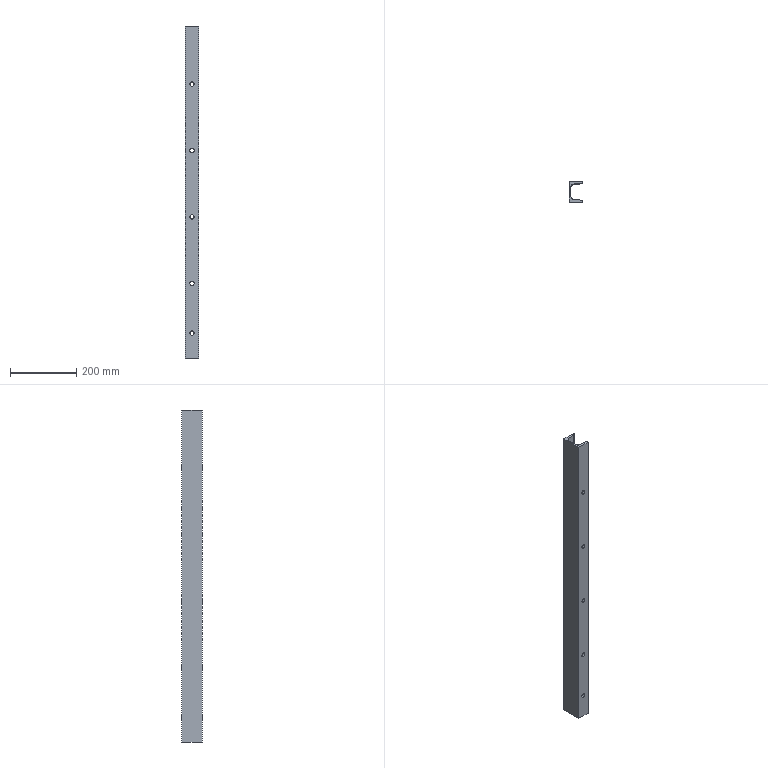Part | SolidWorks | features BaseBody 1 | 1 solid | 34 faces | box 40 x 63 x 1000 mm | volume 834296 mm3 | cylinder 24 | plane 10 | commonest cylinder face diameters 13 x20 7.6 x2 15 x2
STEP:
#1=CARTESIAN_POINT('',(12.9,-31.5,825.));
#2=VERTEX_POINT('',#1);
#3=CARTESIAN_POINT('',(-0.1,-31.5,825.));
#4=VERTEX_POINT('',#3);
#5=CARTESIAN_POINT('',(6.4,-31.5,825.));
#6=DIRECTION('',(0.,1.,0.));
#7=DIRECTION('',(-1.,0.,0.));
#8=AXIS2_PLACEMENT_3D('',#5,#6,#7);
#9=CIRCLE('',#8,6.5);
#10=EDGE_CURVE('',#2,#4,#9,.T.);
#11=ORIENTED_EDGE('',*,*,#10,.F.);
#12=CARTESIAN_POINT('',(12.9,-24.41,825.));
#13=VERTEX_POINT('',#12);
#14=CARTESIAN_POINT('',(12.9,-971.281,825.));
#15=DIRECTION('',(0.,1.,0.));
#16=VECTOR('',#15,1000.);
#17=LINE('',#14,#16);
#18=EDGE_CURVE('',#2,#13,#17,.T.);
#19=ORIENTED_EDGE('',*,*,#18,.T.);
#20=CARTESIAN_POINT('',(-0.1,-23.11,825.));
#21=VERTEX_POINT('',#20);
#22=CARTESIAN_POINT('',(-0.1,-23.11,825.));
#23=CARTESIAN_POINT('',(-0.1,-23.11,812.));
#24=CARTESIAN_POINT('',(12.9,-24.41,812.));
#25=CARTESIAN_POINT('',(12.9,-24.41,825.));
#26=(BOUNDED_CURVE()B_SPLINE_CURVE(3,(#22,#23,#24,#25),.UNSPECIFIED.,.F.,.F.)B_SPLINE_CURVE_WITH_KNOTS((4,4),(0.,3.142),.UNSPECIFIED.)CURVE()GEOMETRIC_REPRESENTATION_ITEM()RATIONAL_B_SPLINE_CURVE((1.,0.3333,0.3333,1.))REPRESENTATION_ITEM(''));
#27=EDGE_CURVE('',#21,#13,#26,.T.);
#28=ORIENTED_EDGE('',*,*,#27,.F.);
#29=CARTESIAN_POINT('',(-0.1,-971.281,825.));
#30=DIRECTION('',(0.,1.,0.));
#31=VECTOR('',#30,1000.);
#32=LINE('',#29,#31);
#33=EDGE_CURVE('',#4,#21,#32,.T.);
#34=ORIENTED_EDGE('',*,*,#33,.F.);
#35=EDGE_LOOP('',(#11,#19,#28,#34));
#36=FACE_OUTER_BOUND('',#35,.T.);
#37=CARTESIAN_POINT('',(6.4,-971.281,825.));
#38=DIRECTION('',(0.,1.,0.));
#39=DIRECTION('',(-1.,0.,0.));
#40=AXIS2_PLACEMENT_3D('',#37,#38,#39);
#41=CYLINDRICAL_SURFACE('',#40,6.5);
#42=ADVANCED_FACE('',(#36),#41,.F.);
#43=CARTESIAN_POINT('',(12.9,-31.5,425.));
#44=VERTEX_POINT('',#43);
#45=CARTESIAN_POINT('',(-0.1,-31.5,425.));
#46=VERTEX_POINT('',#45);
#47=CARTESIAN_POINT('',(6.4,-31.5,425.));
#48=DIRECTION('',(0.,1.,0.));
#49=DIRECTION('',(-1.,0.,0.));
#50=AXIS2_PLACEMENT_3D('',#47,#48,#49);
#51=CIRCLE('',#50,6.5);
#52=EDGE_CURVE('',#44,#46,#51,.T.);
#53=ORIENTED_EDGE('',*,*,#52,.F.);
#54=CARTESIAN_POINT('',(12.9,-24.41,425.));
#55=VERTEX_POINT('',#54);
#56=CARTESIAN_POINT('',(12.9,-971.281,425.));
#57=DIRECTION('',(0.,1.,0.));
#58=VECTOR('',#57,1000.);
#59=LINE('',#56,#58);
#60=EDGE_CURVE('',#44,#55,#59,.T.);
#61=ORIENTED_EDGE('',*,*,#60,.T.);
#62=CARTESIAN_POINT('',(-0.1,-23.11,425.));
#63=VERTEX_POINT('',#62);
#64=CARTESIAN_POINT('',(-0.1,-23.11,425.));
#65=CARTESIAN_POINT('',(-0.1,-23.11,412.));
#66=CARTESIAN_POINT('',(12.9,-24.41,412.));
#67=CARTESIAN_POINT('',(12.9,-24.41,425.));
#68=(BOUNDED_CURVE()B_SPLINE_CURVE(3,(#64,#65,#66,#67),.UNSPECIFIED.,.F.,.F.)B_SPLINE_CURVE_WITH_KNOTS((4,4),(0.,3.142),.UNSPECIFIED.)CURVE()GEOMETRIC_REPRESENTATION_ITEM()RATIONAL_B_SPLINE_CURVE((1.,0.3333,0.3333,1.))REPRESENTATION_ITEM(''));
#69=EDGE_CURVE('',#63,#55,#68,.T.);
#70=ORIENTED_EDGE('',*,*,#69,.F.);
#71=CARTESIAN_POINT('',(-0.1,-971.281,425.));
#72=DIRECTION('',(0.,1.,0.));
#73=VECTOR('',#72,1000.);
#74=LINE('',#71,#73);
#75=EDGE_CURVE('',#46,#63,#74,.T.);
#76=ORIENTED_EDGE('',*,*,#75,.F.);
#77=EDGE_LOOP('',(#53,#61,#70,#76));
#78=FACE_OUTER_BOUND('',#77,.T.);
#79=CARTESIAN_POINT('',(6.4,-971.281,425.));
#80=DIRECTION('',(0.,1.,0.));
#81=DIRECTION('',(-1.,0.,0.));
#82=AXIS2_PLACEMENT_3D('',#79,#80,#81);
#83=CYLINDRICAL_SURFACE('',#82,6.5);
#84=ADVANCED_FACE('',(#78),#83,.F.);
#85=CARTESIAN_POINT('',(12.9,-31.5,75.));
#86=VERTEX_POINT('',#85);
#87=CARTESIAN_POINT('',(-0.1,-31.5,75.));
#88=VERTEX_POINT('',#87);
#89=CARTESIAN_POINT('',(6.4,-31.5,75.));
#90=DIRECTION('',(0.,1.,0.));
#91=DIRECTION('',(-1.,0.,0.));
#92=AXIS2_PLACEMENT_3D('',#89,#90,#91);
#93=CIRCLE('',#92,6.5);
#94=EDGE_CURVE('',#86,#88,#93,.T.);
#95=ORIENTED_EDGE('',*,*,#94,.F.);
#96=CARTESIAN_POINT('',(12.9,-24.41,75.));
#97=VERTEX_POINT('',#96);
#98=CARTESIAN_POINT('',(12.9,-971.281,75.));
#99=DIRECTION('',(0.,1.,0.));
#100=VECTOR('',#99,1000.);
#101=LINE('',#98,#100);
#102=EDGE_CURVE('',#86,#97,#101,.T.);
#103=ORIENTED_EDGE('',*,*,#102,.T.);
#104=CARTESIAN_POINT('',(-0.1,-23.11,75.));
#105=VERTEX_POINT('',#104);
#106=CARTESIAN_POINT('',(-0.1,-23.11,75.));
#107=CARTESIAN_POINT('',(-0.1,-23.11,62.));
#108=CARTESIAN_POINT('',(12.9,-24.41,62.));
#109=CARTESIAN_POINT('',(12.9,-24.41,75.));
#110=(BOUNDED_CURVE()B_SPLINE_CURVE(3,(#106,#107,#108,#109),.UNSPECIFIED.,.F.,.F.)B_SPLINE_CURVE_WITH_KNOTS((4,4),(0.,3.142),.UNSPECIFIED.)CURVE()GEOMETRIC_REPRESENTATION_ITEM()RATIONAL_B_SPLINE_CURVE((1.,0.3333,0.3333,1.))REPRESENTATION_ITEM(''));
#111=EDGE_CURVE('',#105,#97,#110,.T.);
#112=ORIENTED_EDGE('',*,*,#111,.F.);
#113=CARTESIAN_POINT('',(-0.1,-971.281,75.));
#114=DIRECTION('',(0.,1.,0.));
#115=VECTOR('',#114,1000.);
#116=LINE('',#113,#115);
#117=EDGE_CURVE('',#88,#105,#116,.T.);
#118=ORIENTED_EDGE('',*,*,#117,.F.);
#119=EDGE_LOOP('',(#95,#103,#112,#118));
#120=FACE_OUTER_BOUND('',#119,.T.);
#121=CARTESIAN_POINT('',(6.4,-971.281,75.));
#122=DIRECTION('',(0.,1.,0.));
#123=DIRECTION('',(-1.,0.,0.));
#124=AXIS2_PLACEMENT_3D('',#121,#122,#123);
#125=CYLINDRICAL_SURFACE('',#124,6.5);
#126=ADVANCED_FACE('',(#120),#125,.F.);
#127=CARTESIAN_POINT('',(12.9,-31.5,225.));
#128=VERTEX_POINT('',#127);
#129=CARTESIAN_POINT('',(-0.1,-31.5,225.));
#130=VERTEX_POINT('',#129);
#131=CARTESIAN_POINT('',(6.4,-31.5,225.));
#132=DIRECTION('',(0.,1.,0.));
#133=DIRECTION('',(-1.,0.,0.));
#134=AXIS2_PLACEMENT_3D('',#131,#132,#133);
#135=CIRCLE('',#134,6.5);
#136=EDGE_CURVE('',#128,#130,#135,.T.);
#137=ORIENTED_EDGE('',*,*,#136,.F.);
#138=CARTESIAN_POINT('',(12.9,-24.41,225.));
#139=VERTEX_POINT('',#138);
#140=CARTESIAN_POINT('',(12.9,-971.281,225.));
#141=DIRECTION('',(0.,1.,0.));
#142=VECTOR('',#141,1000.);
#143=LINE('',#140,#142);
#144=EDGE_CURVE('',#128,#139,#143,.T.);
#145=ORIENTED_EDGE('',*,*,#144,.T.);
#146=CARTESIAN_POINT('',(-0.1,-23.11,225.));
#147=VERTEX_POINT('',#146);
#148=CARTESIAN_POINT('',(-0.1,-23.11,225.));
#149=CARTESIAN_POINT('',(-0.1,-23.11,212.));
#150=CARTESIAN_POINT('',(12.9,-24.41,212.));
#151=CARTESIAN_POINT('',(12.9,-24.41,225.));
#152=(BOUNDED_CURVE()B_SPLINE_CURVE(3,(#148,#149,#150,#151),.UNSPECIFIED.,.F.,.T.)B_SPLINE_CURVE_WITH_KNOTS((4,4),(0.,3.142),.UNSPECIFIED.)CURVE()GEOMETRIC_REPRESENTATION_ITEM()RATIONAL_B_SPLINE_CURVE((1.,0.3333,0.3333,1.))REPRESENTATION_ITEM(''));
#153=EDGE_CURVE('',#147,#139,#152,.T.);
#154=ORIENTED_EDGE('',*,*,#153,.F.);
#155=CARTESIAN_POINT('',(-0.1,-971.281,225.));
#156=DIRECTION('',(0.,1.,0.));
#157=VECTOR('',#156,1000.);
#158=LINE('',#155,#157);
#159=EDGE_CURVE('',#130,#147,#158,.T.);
#160=ORIENTED_EDGE('',*,*,#159,.F.);
#161=EDGE_LOOP('',(#137,#145,#154,#160));
#162=FACE_OUTER_BOUND('',#161,.T.);
#163=CARTESIAN_POINT('',(6.4,-971.281,225.));
#164=DIRECTION('',(0.,1.,0.));
#165=DIRECTION('',(-1.,0.,0.));
#166=AXIS2_PLACEMENT_3D('',#163,#164,#165);
#167=CYLINDRICAL_SURFACE('',#166,6.5);
#168=ADVANCED_FACE('',(#162),#167,.F.);
#169=CARTESIAN_POINT('',(12.9,-31.5,625.));
#170=VERTEX_POINT('',#169);
#171=CARTESIAN_POINT('',(-0.1,-31.5,625.));
#172=VERTEX_POINT('',#171);
#173=CARTESIAN_POINT('',(6.4,-31.5,625.));
#174=DIRECTION('',(0.,1.,0.));
#175=DIRECTION('',(-1.,0.,0.));
#176=AXIS2_PLACEMENT_3D('',#173,#174,#175);
#177=CIRCLE('',#176,6.5);
#178=EDGE_CURVE('',#170,#172,#177,.T.);
#179=ORIENTED_EDGE('',*,*,#178,.F.);
#180=CARTESIAN_POINT('',(12.9,-24.41,625.));
#181=VERTEX_POINT('',#180);
#182=CARTESIAN_POINT('',(12.9,-971.281,625.));
#183=DIRECTION('',(0.,1.,0.));
#184=VECTOR('',#183,1000.);
#185=LINE('',#182,#184);
#186=EDGE_CURVE('',#170,#181,#185,.T.);
#187=ORIENTED_EDGE('',*,*,#186,.T.);
#188=CARTESIAN_POINT('',(-0.1,-23.11,625.));
#189=VERTEX_POINT('',#188);
#190=CARTESIAN_POINT('',(-0.1,-23.11,625.));
#191=CARTESIAN_POINT('',(-0.1,-23.11,612.));
#192=CARTESIAN_POINT('',(12.9,-24.41,612.));
#193=CARTESIAN_POINT('',(12.9,-24.41,625.));
#194=(BOUNDED_CURVE()B_SPLINE_CURVE(3,(#190,#191,#192,#193),.UNSPECIFIED.,.F.,.F.)B_SPLINE_CURVE_WITH_KNOTS((4,4),(0.,3.142),.UNSPECIFIED.)CURVE()GEOMETRIC_REPRESENTATION_ITEM()RATIONAL_B_SPLINE_CURVE((1.,0.3333,0.3333,1.))REPRESENTATION_ITEM(''));
#195=EDGE_CURVE('',#189,#181,#194,.T.);
#196=ORIENTED_EDGE('',*,*,#195,.F.);
#197=CARTESIAN_POINT('',(-0.1,-971.281,625.));
#198=DIRECTION('',(0.,1.,0.));
#199=VECTOR('',#198,1000.);
#200=LINE('',#197,#199);
#201=EDGE_CURVE('',#172,#189,#200,.T.);
#202=ORIENTED_EDGE('',*,*,#201,.F.);
#203=EDGE_LOOP('',(#179,#187,#196,#202));
#204=FACE_OUTER_BOUND('',#203,.T.);
#205=CARTESIAN_POINT('',(6.4,-971.281,625.));
#206=DIRECTION('',(0.,1.,0.));
#207=DIRECTION('',(-1.,0.,0.));
#208=AXIS2_PLACEMENT_3D('',#205,#206,#207);
#209=CYLINDRICAL_SURFACE('',#208,6.5);
#210=ADVANCED_FACE('',(#204),#209,.F.);
#211=CARTESIAN_POINT('',(12.9,24.41,825.));
#212=VERTEX_POINT('',#211);
#213=CARTESIAN_POINT('',(-0.1,23.11,825.));
#214=VERTEX_POINT('',#213);
#215=CARTESIAN_POINT('',(12.9,24.41,825.));
#216=CARTESIAN_POINT('',(12.9,24.41,812.));
#217=CARTESIAN_POINT('',(-0.1,23.11,812.));
#218=CARTESIAN_POINT('',(-0.1,23.11,825.));
#219=(BOUNDED_CURVE()B_SPLINE_CURVE(3,(#215,#216,#217,#218),.UNSPECIFIED.,.F.,.T.)B_SPLINE_CURVE_WITH_KNOTS((4,4),(0.,3.142),.UNSPECIFIED.)CURVE()GEOMETRIC_REPRESENTATION_ITEM()RATIONAL_B_SPLINE_CURVE((1.,0.3333,0.3333,1.))REPRESENTATION_ITEM(''));
#220=EDGE_CURVE('',#212,#214,#219,.T.);
#221=ORIENTED_EDGE('',*,*,#220,.F.);
#222=CARTESIAN_POINT('',(12.9,31.5,825.));
#223=VERTEX_POINT('',#222);
#224=CARTESIAN_POINT('',(12.9,-971.281,825.));
#225=DIRECTION('',(0.,1.,0.));
#226=VECTOR('',#225,1000.);
#227=LINE('',#224,#226);
#228=EDGE_CURVE('',#212,#223,#227,.T.);
#229=ORIENTED_EDGE('',*,*,#228,.T.);
#230=CARTESIAN_POINT('',(-0.1,31.5,825.));
#231=VERTEX_POINT('',#230);
#232=CARTESIAN_POINT('',(6.4,31.5,825.));
#233=DIRECTION('',(0.,-1.,0.));
#234=DIRECTION('',(-1.,0.,0.));
#235=AXIS2_PLACEMENT_3D('',#232,#233,#234);
#236=CIRCLE('',#235,6.5);
#237=EDGE_CURVE('',#231,#223,#236,.T.);
#238=ORIENTED_EDGE('',*,*,#237,.F.);
#239=CARTESIAN_POINT('',(-0.1,-971.281,825.));
#240=DIRECTION('',(0.,1.,0.));
#241=VECTOR('',#240,1000.);
#242=LINE('',#239,#241);
#243=EDGE_CURVE('',#214,#231,#242,.T.);
#244=ORIENTED_EDGE('',*,*,#243,.F.);
#245=EDGE_LOOP('',(#221,#229,#238,#244));
#246=FACE_OUTER_BOUND('',#245,.T.);
#247=CARTESIAN_POINT('',(6.4,-971.281,825.));
#248=DIRECTION('',(0.,1.,0.));
#249=DIRECTION('',(-1.,0.,0.));
#250=AXIS2_PLACEMENT_3D('',#247,#248,#249);
#251=CYLINDRICAL_SURFACE('',#250,6.5);
#252=ADVANCED_FACE('',(#246),#251,.F.);
#253=CARTESIAN_POINT('',(12.9,24.41,425.));
#254=VERTEX_POINT('',#253);
#255=CARTESIAN_POINT('',(-0.1,23.11,425.));
#256=VERTEX_POINT('',#255);
#257=CARTESIAN_POINT('',(12.9,24.41,425.));
#258=CARTESIAN_POINT('',(12.9,24.41,412.));
#259=CARTESIAN_POINT('',(-0.1,23.11,412.));
#260=CARTESIAN_POINT('',(-0.1,23.11,425.));
#261=(BOUNDED_CURVE()B_SPLINE_CURVE(3,(#257,#258,#259,#260),.UNSPECIFIED.,.F.,.T.)B_SPLINE_CURVE_WITH_KNOTS((4,4),(0.,3.142),.UNSPECIFIED.)CURVE()GEOMETRIC_REPRESENTATION_ITEM()RATIONAL_B_SPLINE_CURVE((1.,0.3333,0.3333,1.))REPRESENTATION_ITEM(''));
#262=EDGE_CURVE('',#254,#256,#261,.T.);
#263=ORIENTED_EDGE('',*,*,#262,.F.);
#264=CARTESIAN_POINT('',(12.9,31.5,425.));
#265=VERTEX_POINT('',#264);
#266=CARTESIAN_POINT('',(12.9,-971.281,425.));
#267=DIRECTION('',(0.,1.,0.));
#268=VECTOR('',#267,1000.);
#269=LINE('',#266,#268);
#270=EDGE_CURVE('',#254,#265,#269,.T.);
#271=ORIENTED_EDGE('',*,*,#270,.T.);
#272=CARTESIAN_POINT('',(-0.1,31.5,425.));
#273=VERTEX_POINT('',#272);
#274=CARTESIAN_POINT('',(6.4,31.5,425.));
#275=DIRECTION('',(0.,-1.,0.));
#276=DIRECTION('',(-1.,0.,0.));
#277=AXIS2_PLACEMENT_3D('',#274,#275,#276);
#278=CIRCLE('',#277,6.5);
#279=EDGE_CURVE('',#273,#265,#278,.T.);
#280=ORIENTED_EDGE('',*,*,#279,.F.);
#281=CARTESIAN_POINT('',(-0.1,-971.281,425.));
#282=DIRECTION('',(0.,1.,0.));
#283=VECTOR('',#282,1000.);
#284=LINE('',#281,#283);
#285=EDGE_CURVE('',#256,#273,#284,.T.);
#286=ORIENTED_EDGE('',*,*,#285,.F.);
#287=EDGE_LOOP('',(#263,#271,#280,#286));
#288=FACE_OUTER_BOUND('',#287,.T.);
#289=CARTESIAN_POINT('',(6.4,-971.281,425.));
#290=DIRECTION('',(0.,1.,0.));
#291=DIRECTION('',(-1.,0.,0.));
#292=AXIS2_PLACEMENT_3D('',#289,#290,#291);
#293=CYLINDRICAL_SURFACE('',#292,6.5);
#294=ADVANCED_FACE('',(#288),#293,.F.);
#295=CARTESIAN_POINT('',(12.9,24.41,75.));
#296=VERTEX_POINT('',#295);
#297=CARTESIAN_POINT('',(-0.1,23.11,75.));
#298=VERTEX_POINT('',#297);
#299=CARTESIAN_POINT('',(12.9,24.41,75.));
#300=CARTESIAN_POINT('',(12.9,24.41,62.));
#301=CARTESIAN_POINT('',(-0.1,23.11,62.));
#302=CARTESIAN_POINT('',(-0.1,23.11,75.));
#303=(BOUNDED_CURVE()B_SPLINE_CURVE(3,(#299,#300,#301,#302),.UNSPECIFIED.,.F.,.F.)B_SPLINE_CURVE_WITH_KNOTS((4,4),(0.,3.142),.UNSPECIFIED.)CURVE()GEOMETRIC_REPRESENTATION_ITEM()RATIONAL_B_SPLINE_CURVE((1.,0.3333,0.3333,1.))REPRESENTATION_ITEM(''));
#304=EDGE_CURVE('',#296,#298,#303,.T.);
#305=ORIENTED_EDGE('',*,*,#304,.F.);
#306=CARTESIAN_POINT('',(12.9,31.5,75.));
#307=VERTEX_POINT('',#306);
#308=CARTESIAN_POINT('',(12.9,-971.281,75.));
#309=DIRECTION('',(0.,1.,0.));
#310=VECTOR('',#309,1000.);
#311=LINE('',#308,#310);
#312=EDGE_CURVE('',#296,#307,#311,.T.);
#313=ORIENTED_EDGE('',*,*,#312,.T.);
#314=CARTESIAN_POINT('',(-0.1,31.5,75.));
#315=VERTEX_POINT('',#314);
#316=CARTESIAN_POINT('',(6.4,31.5,75.));
#317=DIRECTION('',(0.,-1.,0.));
#318=DIRECTION('',(-1.,0.,0.));
#319=AXIS2_PLACEMENT_3D('',#316,#317,#318);
#320=CIRCLE('',#319,6.5);
#321=EDGE_CURVE('',#315,#307,#320,.T.);
#322=ORIENTED_EDGE('',*,*,#321,.F.);
#323=CARTESIAN_POINT('',(-0.1,-971.281,75.));
#324=DIRECTION('',(0.,1.,0.));
#325=VECTOR('',#324,1000.);
#326=LINE('',#323,#325);
#327=EDGE_CURVE('',#298,#315,#326,.T.);
#328=ORIENTED_EDGE('',*,*,#327,.F.);
#329=EDGE_LOOP('',(#305,#313,#322,#328));
#330=FACE_OUTER_BOUND('',#329,.T.);
#331=CARTESIAN_POINT('',(6.4,-971.281,75.));
#332=DIRECTION('',(0.,1.,0.));
#333=DIRECTION('',(-1.,0.,0.));
#334=AXIS2_PLACEMENT_3D('',#331,#332,#333);
#335=CYLINDRICAL_SURFACE('',#334,6.5);
#336=ADVANCED_FACE('',(#330),#335,.F.);
#337=CARTESIAN_POINT('',(12.9,24.41,225.));
#338=VERTEX_POINT('',#337);
#339=CARTESIAN_POINT('',(-0.1,23.11,225.));
#340=VERTEX_POINT('',#339);
#341=CARTESIAN_POINT('',(12.9,24.41,225.));
#342=CARTESIAN_POINT('',(12.9,24.41,212.));
#343=CARTESIAN_POINT('',(-0.1,23.11,212.));
#344=CARTESIAN_POINT('',(-0.1,23.11,225.));
#345=(BOUNDED_CURVE()B_SPLINE_CURVE(3,(#341,#342,#343,#344),.UNSPECIFIED.,.F.,.T.)B_SPLINE_CURVE_WITH_KNOTS((4,4),(0.,3.142),.UNSPECIFIED.)CURVE()GEOMETRIC_REPRESENTATION_ITEM()RATIONAL_B_SPLINE_CURVE((1.,0.3333,0.3333,1.))REPRESENTATION_ITEM(''));
#346=EDGE_CURVE('',#338,#340,#345,.T.);
#347=ORIENTED_EDGE('',*,*,#346,.F.);
#348=CARTESIAN_POINT('',(12.9,31.5,225.));
#349=VERTEX_POINT('',#348);
#350=CARTESIAN_POINT('',(12.9,-971.281,225.));
#351=DIRECTION('',(0.,1.,0.));
#352=VECTOR('',#351,1000.);
#353=LINE('',#350,#352);
#354=EDGE_CURVE('',#338,#349,#353,.T.);
#355=ORIENTED_EDGE('',*,*,#354,.T.);
#356=CARTESIAN_POINT('',(-0.1,31.5,225.));
#357=VERTEX_POINT('',#356);
#358=CARTESIAN_POINT('',(6.4,31.5,225.));
#359=DIRECTION('',(0.,-1.,0.));
#360=DIRECTION('',(-1.,0.,0.));
#361=AXIS2_PLACEMENT_3D('',#358,#359,#360);
#362=CIRCLE('',#361,6.5);
#363=EDGE_CURVE('',#357,#349,#362,.T.);
#364=ORIENTED_EDGE('',*,*,#363,.F.);
#365=CARTESIAN_POINT('',(-0.1,-971.281,225.));
#366=DIRECTION('',(0.,1.,0.));
#367=VECTOR('',#366,1000.);
#368=LINE('',#365,#367);
#369=EDGE_CURVE('',#340,#357,#368,.T.);
#370=ORIENTED_EDGE('',*,*,#369,.F.);
#371=EDGE_LOOP('',(#347,#355,#364,#370));
#372=FACE_OUTER_BOUND('',#371,.T.);
#373=CARTESIAN_POINT('',(6.4,-971.281,225.));
#374=DIRECTION('',(0.,1.,0.));
#375=DIRECTION('',(-1.,0.,0.));
#376=AXIS2_PLACEMENT_3D('',#373,#374,#375);
#377=CYLINDRICAL_SURFACE('',#376,6.5);
#378=ADVANCED_FACE('',(#372),#377,.F.);
#379=CARTESIAN_POINT('',(12.9,24.41,625.));
#380=VERTEX_POINT('',#379);
#381=CARTESIAN_POINT('',(-0.1,23.11,625.));
#382=VERTEX_POINT('',#381);
#383=CARTESIAN_POINT('',(12.9,24.41,625.));
#384=CARTESIAN_POINT('',(12.9,24.41,612.));
#385=CARTESIAN_POINT('',(-0.1,23.11,612.));
#386=CARTESIAN_POINT('',(-0.1,23.11,625.));
#387=(BOUNDED_CURVE()B_SPLINE_CURVE(3,(#383,#384,#385,#386),.UNSPECIFIED.,.F.,.F.)B_SPLINE_CURVE_WITH_KNOTS((4,4),(0.,3.142),.UNSPECIFIED.)CURVE()GEOMETRIC_REPRESENTATION_ITEM()RATIONAL_B_SPLINE_CURVE((1.,0.3333,0.3333,1.))REPRESENTATION_ITEM(''));
#388=EDGE_CURVE('',#380,#382,#387,.T.);
#389=ORIENTED_EDGE('',*,*,#388,.F.);
#390=CARTESIAN_POINT('',(12.9,31.5,625.));
#391=VERTEX_POINT('',#390);
#392=CARTESIAN_POINT('',(12.9,-971.281,625.));
#393=DIRECTION('',(0.,1.,0.));
#394=VECTOR('',#393,1000.);
#395=LINE('',#392,#394);
#396=EDGE_CURVE('',#380,#391,#395,.T.);
#397=ORIENTED_EDGE('',*,*,#396,.T.);
#398=CARTESIAN_POINT('',(-0.1,31.5,625.));
#399=VERTEX_POINT('',#398);
#400=CARTESIAN_POINT('',(6.4,31.5,625.));
#401=DIRECTION('',(0.,-1.,0.));
#402=DIRECTION('',(-1.,0.,0.));
#403=AXIS2_PLACEMENT_3D('',#400,#401,#402);
#404=CIRCLE('',#403,6.5);
#405=EDGE_CURVE('',#399,#391,#404,.T.);
#406=ORIENTED_EDGE('',*,*,#405,.F.);
#407=CARTESIAN_POINT('',(-0.1,-971.281,625.));
#408=DIRECTION('',(0.,1.,0.));
#409=VECTOR('',#408,1000.);
#410=LINE('',#407,#409);
#411=EDGE_CURVE('',#382,#399,#410,.T.);
#412=ORIENTED_EDGE('',*,*,#411,.F.);
#413=EDGE_LOOP('',(#389,#397,#406,#412));
#414=FACE_OUTER_BOUND('',#413,.T.);
#415=CARTESIAN_POINT('',(6.4,-971.281,625.));
#416=DIRECTION('',(0.,1.,0.));
#417=DIRECTION('',(-1.,0.,0.));
#418=AXIS2_PLACEMENT_3D('',#415,#416,#417);
#419=CYLINDRICAL_SURFACE('',#418,6.5);
#420=ADVANCED_FACE('',(#414),#419,.F.);
#421=CARTESIAN_POINT('',(-13.6,31.5,0.));
#422=VERTEX_POINT('',#421);
#423=CARTESIAN_POINT('',(-13.6,-31.5,0.));
#424=VERTEX_POINT('',#423);
#425=CARTESIAN_POINT('',(-13.6,0.,0.));
#426=DIRECTION('',(0.,-1.,0.));
#427=VECTOR('',#426,1000.);
#428=LINE('',#425,#427);
#429=EDGE_CURVE('',#422,#424,#428,.T.);
#430=ORIENTED_EDGE('',*,*,#429,.T.);
#431=CARTESIAN_POINT('',(-13.6,-31.5,1000.));
#432=VERTEX_POINT('',#431);
#433=CARTESIAN_POINT('',(-13.6,-31.5,0.));
#434=DIRECTION('',(0.,0.,1.));
#435=VECTOR('',#434,1000.);
#436=LINE('',#433,#435);
#437=EDGE_CURVE('',#424,#432,#436,.T.);
#438=ORIENTED_EDGE('',*,*,#437,.T.);
#439=CARTESIAN_POINT('',(-13.6,31.5,1000.));
#440=VERTEX_POINT('',#439);
#441=CARTESIAN_POINT('',(-13.6,0.,1000.));
#442=DIRECTION('',(0.,1.,0.));
#443=VECTOR('',#442,1000.);
#444=LINE('',#441,#443);
#445=EDGE_CURVE('',#432,#440,#444,.T.);
#446=ORIENTED_EDGE('',*,*,#445,.T.);
#447=CARTESIAN_POINT('',(-13.6,31.5,0.));
#448=DIRECTION('',(0.,0.,-1.));
#449=VECTOR('',#448,1000.);
#450=LINE('',#447,#449);
#451=EDGE_CURVE('',#440,#422,#450,.T.);
#452=ORIENTED_EDGE('',*,*,#451,.T.);
#453=EDGE_LOOP('',(#430,#438,#446,#452));
#454=FACE_OUTER_BOUND('',#453,.T.);
#455=CARTESIAN_POINT('',(-13.6,0.,0.));
#456=DIRECTION('',(-1.,0.,0.));
#457=DIRECTION('',(0.,-1.,0.));
#458=AXIS2_PLACEMENT_3D('',#455,#456,#457);
#459=PLANE('',#458);
#460=ADVANCED_FACE('',(#454),#459,.T.);
#461=CARTESIAN_POINT('',(6.4,-31.5,825.));
#462=DIRECTION('',(0.,1.,0.));
#463=DIRECTION('',(-1.,0.,0.));
#464=AXIS2_PLACEMENT_3D('',#461,#462,#463);
#465=CIRCLE('',#464,6.5);
#466=EDGE_CURVE('',#4,#2,#465,.T.);
#467=ORIENTED_EDGE('',*,*,#466,.T.);
#468=ORIENTED_EDGE('',*,*,#10,.T.);
#469=EDGE_LOOP('',(#467,#468));
#470=FACE_BOUND('',#469,.T.);
#471=CARTESIAN_POINT('',(6.4,-31.5,425.));
#472=DIRECTION('',(0.,1.,0.));
#473=DIRECTION('',(-1.,0.,0.));
#474=AXIS2_PLACEMENT_3D('',#471,#472,#473);
#475=CIRCLE('',#474,6.5);
#476=EDGE_CURVE('',#46,#44,#475,.T.);
#477=ORIENTED_EDGE('',*,*,#476,.T.);
#478=ORIENTED_EDGE('',*,*,#52,.T.);
#479=EDGE_LOOP('',(#477,#478));
#480=FACE_BOUND('',#479,.T.);
#481=CARTESIAN_POINT('',(6.4,-31.5,75.));
#482=DIRECTION('',(0.,1.,0.));
#483=DIRECTION('',(-1.,0.,0.));
#484=AXIS2_PLACEMENT_3D('',#481,#482,#483);
#485=CIRCLE('',#484,6.5);
#486=EDGE_CURVE('',#88,#86,#485,.T.);
#487=ORIENTED_EDGE('',*,*,#486,.T.);
#488=ORIENTED_EDGE('',*,*,#94,.T.);
#489=EDGE_LOOP('',(#487,#488));
#490=FACE_BOUND('',#489,.T.);
#491=CARTESIAN_POINT('',(6.4,-31.5,225.));
#492=DIRECTION('',(0.,1.,0.));
#493=DIRECTION('',(-1.,0.,0.));
#494=AXIS2_PLACEMENT_3D('',#491,#492,#493);
#495=CIRCLE('',#494,6.5);
#496=EDGE_CURVE('',#130,#128,#495,.T.);
#497=ORIENTED_EDGE('',*,*,#496,.T.);
#498=ORIENTED_EDGE('',*,*,#136,.T.);
#499=EDGE_LOOP('',(#497,#498));
#500=FACE_BOUND('',#499,.T.);
#501=CARTESIAN_POINT('',(6.4,-31.5,625.));
#502=DIRECTION('',(0.,1.,0.));
#503=DIRECTION('',(-1.,0.,0.));
#504=AXIS2_PLACEMENT_3D('',#501,#502,#503);
#505=CIRCLE('',#504,6.5);
#506=EDGE_CURVE('',#172,#170,#505,.T.);
#507=ORIENTED_EDGE('',*,*,#506,.T.);
#508=ORIENTED_EDGE('',*,*,#178,.T.);
#509=EDGE_LOOP('',(#507,#508));
#510=FACE_BOUND('',#509,.T.);
#511=CARTESIAN_POINT('',(26.4,-31.5,0.));
#512=VERTEX_POINT('',#511);
#513=CARTESIAN_POINT('',(26.4,-31.5,0.));
#514=DIRECTION('',(1.,0.,0.));
#515=VECTOR('',#514,1000.);
#516=LINE('',#513,#515);
#517=EDGE_CURVE('',#424,#512,#516,.T.);
#518=ORIENTED_EDGE('',*,*,#517,.T.);
#519=CARTESIAN_POINT('',(26.4,-31.5,1000.));
#520=VERTEX_POINT('',#519);
#521=CARTESIAN_POINT('',(26.4,-31.5,0.));
#522=DIRECTION('',(0.,0.,1.));
#523=VECTOR('',#522,1000.);
#524=LINE('',#521,#523);
#525=EDGE_CURVE('',#512,#520,#524,.T.);
#526=ORIENTED_EDGE('',*,*,#525,.T.);
#527=CARTESIAN_POINT('',(26.4,-31.5,1000.));
#528=DIRECTION('',(-1.,0.,0.));
#529=VECTOR('',#528,1000.);
#530=LINE('',#527,#529);
#531=EDGE_CURVE('',#520,#432,#530,.T.);
#532=ORIENTED_EDGE('',*,*,#531,.T.);
#533=ORIENTED_EDGE('',*,*,#437,.F.);
#534=EDGE_LOOP('',(#518,#526,#532,#533));
#535=FACE_OUTER_BOUND('',#534,.T.);
#536=CARTESIAN_POINT('',(26.4,-31.5,0.));
#537=DIRECTION('',(0.,-1.,0.));
#538=DIRECTION('',(0.,0.,-1.));
#539=AXIS2_PLACEMENT_3D('',#536,#537,#538);
#540=PLANE('',#539);
#541=ADVANCED_FACE('',(#470,#480,#490,#500,#510,#535),#540,.T.);
#542=CARTESIAN_POINT('',(26.4,29.199,0.));
#543=VERTEX_POINT('',#542);
#544=CARTESIAN_POINT('',(26.4,31.5,0.));
#545=VERTEX_POINT('',#544);
#546=CARTESIAN_POINT('',(26.4,0.,0.));
#547=DIRECTION('',(0.,1.,0.));
#548=VECTOR('',#547,1000.);
#549=LINE('',#546,#548);
#550=EDGE_CURVE('',#543,#545,#549,.T.);
#551=ORIENTED_EDGE('',*,*,#550,.F.);
#552=CARTESIAN_POINT('',(22.978,25.418,0.));
#553=VERTEX_POINT('',#552);
#554=CARTESIAN_POINT('',(22.6,29.199,0.));
#555=DIRECTION('',(0.,0.,1.));
#556=DIRECTION('',(1.,0.,0.));
#557=AXIS2_PLACEMENT_3D('',#554,#555,#556);
#558=CIRCLE('',#557,3.8);
#559=EDGE_CURVE('',#553,#543,#558,.T.);
#560=ORIENTED_EDGE('',*,*,#559,.F.);
#561=CARTESIAN_POINT('',(-2.046,22.915,0.));
#562=VERTEX_POINT('',#561);
#563=CARTESIAN_POINT('',(-2.046,22.915,0.));
#564=DIRECTION('',(0.995,0.0995,0.));
#565=VECTOR('',#564,1000.);
#566=LINE('',#563,#565);
#567=EDGE_CURVE('',#562,#553,#566,.T.);
#568=ORIENTED_EDGE('',*,*,#567,.F.);
#569=CARTESIAN_POINT('',(-8.8,15.453,0.));
#570=VERTEX_POINT('',#569);
#571=CARTESIAN_POINT('',(-1.3,15.453,0.));
#572=DIRECTION('',(0.,0.,-1.));
#573=DIRECTION('',(1.,0.,0.));
#574=AXIS2_PLACEMENT_3D('',#571,#572,#573);
#575=CIRCLE('',#574,7.5);
#576=EDGE_CURVE('',#570,#562,#575,.T.);
#577=ORIENTED_EDGE('',*,*,#576,.F.);
#578=CARTESIAN_POINT('',(-8.8,-15.453,0.));
#579=VERTEX_POINT('',#578);
#580=CARTESIAN_POINT('',(-8.8,0.,0.));
#581=DIRECTION('',(0.,1.,0.));
#582=VECTOR('',#581,1000.);
#583=LINE('',#580,#582);
#584=EDGE_CURVE('',#579,#570,#583,.T.);
#585=ORIENTED_EDGE('',*,*,#584,.F.);
#586=CARTESIAN_POINT('',(-2.046,-22.915,0.));
#587=VERTEX_POINT('',#586);
#588=CARTESIAN_POINT('',(-1.3,-15.453,0.));
#589=DIRECTION('',(0.,0.,-1.));
#590=DIRECTION('',(1.,0.,0.));
#591=AXIS2_PLACEMENT_3D('',#588,#589,#590);
#592=CIRCLE('',#591,7.5);
#593=EDGE_CURVE('',#587,#579,#592,.T.);
#594=ORIENTED_EDGE('',*,*,#593,.F.);
#595=CARTESIAN_POINT('',(22.978,-25.418,0.));
#596=VERTEX_POINT('',#595);
#597=CARTESIAN_POINT('',(22.978,-25.418,0.));
#598=DIRECTION('',(-0.995,0.0995,0.));
#599=VECTOR('',#598,1000.);
#600=LINE('',#597,#599);
#601=EDGE_CURVE('',#596,#587,#600,.T.);
#602=ORIENTED_EDGE('',*,*,#601,.F.);
#603=CARTESIAN_POINT('',(26.4,-29.199,0.));
#604=VERTEX_POINT('',#603);
#605=CARTESIAN_POINT('',(22.6,-29.199,0.));
#606=DIRECTION('',(0.,0.,1.));
#607=DIRECTION('',(1.,0.,0.));
#608=AXIS2_PLACEMENT_3D('',#605,#606,#607);
#609=CIRCLE('',#608,3.8);
#610=EDGE_CURVE('',#604,#596,#609,.T.);
#611=ORIENTED_EDGE('',*,*,#610,.F.);
#612=CARTESIAN_POINT('',(26.4,0.,0.));
#613=DIRECTION('',(0.,1.,0.));
#614=VECTOR('',#613,1000.);
#615=LINE('',#612,#614);
#616=EDGE_CURVE('',#512,#604,#615,.T.);
#617=ORIENTED_EDGE('',*,*,#616,.F.);
#618=ORIENTED_EDGE('',*,*,#517,.F.);
#619=ORIENTED_EDGE('',*,*,#429,.F.);
#620=CARTESIAN_POINT('',(6.4,31.5,0.));
#621=DIRECTION('',(-1.,0.,0.));
#622=VECTOR('',#621,1000.);
#623=LINE('',#620,#622);
#624=EDGE_CURVE('',#545,#422,#623,.T.);
#625=ORIENTED_EDGE('',*,*,#624,.F.);
#626=EDGE_LOOP('',(#551,#560,#568,#577,#585,#594,#602,#611,#617,#618,#619,#625));
#627=FACE_OUTER_BOUND('',#626,.T.);
#628=CARTESIAN_POINT('',(6.4,0.,0.));
#629=DIRECTION('',(0.,0.,1.));
#630=DIRECTION('',(1.,0.,0.));
#631=AXIS2_PLACEMENT_3D('',#628,#629,#630);
#632=PLANE('',#631);
#633=ADVANCED_FACE('',(#627),#632,.F.);
#634=ORIENTED_EDGE('',*,*,#237,.T.);
#635=CARTESIAN_POINT('',(6.4,31.5,825.));
#636=DIRECTION('',(0.,-1.,0.));
#637=DIRECTION('',(-1.,0.,0.));
#638=AXIS2_PLACEMENT_3D('',#635,#636,#637);
#639=CIRCLE('',#638,6.5);
#640=EDGE_CURVE('',#223,#231,#639,.T.);
#641=ORIENTED_EDGE('',*,*,#640,.T.);
#642=EDGE_LOOP('',(#634,#641));
#643=FACE_BOUND('',#642,.T.);
#644=ORIENTED_EDGE('',*,*,#279,.T.);
#645=CARTESIAN_POINT('',(6.4,31.5,425.));
#646=DIRECTION('',(0.,-1.,0.));
#647=DIRECTION('',(-1.,0.,0.));
#648=AXIS2_PLACEMENT_3D('',#645,#646,#647);
#649=CIRCLE('',#648,6.5);
#650=EDGE_CURVE('',#265,#273,#649,.T.);
#651=ORIENTED_EDGE('',*,*,#650,.T.);
#652=EDGE_LOOP('',(#644,#651));
#653=FACE_BOUND('',#652,.T.);
#654=ORIENTED_EDGE('',*,*,#321,.T.);
#655=CARTESIAN_POINT('',(6.4,31.5,75.));
#656=DIRECTION('',(0.,-1.,0.));
#657=DIRECTION('',(-1.,0.,0.));
#658=AXIS2_PLACEMENT_3D('',#655,#656,#657);
#659=CIRCLE('',#658,6.5);
#660=EDGE_CURVE('',#307,#315,#659,.T.);
#661=ORIENTED_EDGE('',*,*,#660,.T.);
#662=EDGE_LOOP('',(#654,#661));
#663=FACE_BOUND('',#662,.T.);
#664=ORIENTED_EDGE('',*,*,#363,.T.);
#665=CARTESIAN_POINT('',(6.4,31.5,225.));
#666=DIRECTION('',(0.,-1.,0.));
#667=DIRECTION('',(-1.,0.,0.));
#668=AXIS2_PLACEMENT_3D('',#665,#666,#667);
#669=CIRCLE('',#668,6.5);
#670=EDGE_CURVE('',#349,#357,#669,.T.);
#671=ORIENTED_EDGE('',*,*,#670,.T.);
#672=EDGE_LOOP('',(#664,#671));
#673=FACE_BOUND('',#672,.T.);
#674=ORIENTED_EDGE('',*,*,#405,.T.);
#675=CARTESIAN_POINT('',(6.4,31.5,625.));
#676=DIRECTION('',(0.,-1.,0.));
#677=DIRECTION('',(-1.,0.,0.));
#678=AXIS2_PLACEMENT_3D('',#675,#676,#677);
#679=CIRCLE('',#678,6.5);
#680=EDGE_CURVE('',#391,#399,#679,.T.);
#681=ORIENTED_EDGE('',*,*,#680,.T.);
#682=EDGE_LOOP('',(#674,#681));
#683=FACE_BOUND('',#682,.T.);
#684=ORIENTED_EDGE('',*,*,#624,.T.);
#685=ORIENTED_EDGE('',*,*,#451,.F.);
#686=CARTESIAN_POINT('',(26.4,31.5,1000.));
#687=VERTEX_POINT('',#686);
#688=CARTESIAN_POINT('',(-13.6,31.5,1000.));
#689=DIRECTION('',(1.,0.,0.));
#690=VECTOR('',#689,1000.);
#691=LINE('',#688,#690);
#692=EDGE_CURVE('',#440,#687,#691,.T.);
#693=ORIENTED_EDGE('',*,*,#692,.T.);
#694=CARTESIAN_POINT('',(26.4,31.5,0.));
#695=DIRECTION('',(0.,0.,-1.));
#696=VECTOR('',#695,1000.);
#697=LINE('',#694,#696);
#698=EDGE_CURVE('',#687,#545,#697,.T.);
#699=ORIENTED_EDGE('',*,*,#698,.T.);
#700=EDGE_LOOP('',(#684,#685,#693,#699));
#701=FACE_OUTER_BOUND('',#700,.T.);
#702=CARTESIAN_POINT('',(-13.6,31.5,0.));
#703=DIRECTION('',(0.,1.,0.));
#704=DIRECTION('',(-1.,0.,0.));
#705=AXIS2_PLACEMENT_3D('',#702,#703,#704);
#706=PLANE('',#705);
#707=ADVANCED_FACE('',(#643,#653,#663,#673,#683,#701),#706,.T.);
#708=CARTESIAN_POINT('',(22.978,25.418,1000.));
#709=VERTEX_POINT('',#708);
#710=CARTESIAN_POINT('',(26.4,29.199,1000.));
#711=VERTEX_POINT('',#710);
#712=CARTESIAN_POINT('',(22.6,29.199,1000.));
#713=DIRECTION('',(0.,0.,1.));
#714=DIRECTION('',(1.,0.,0.));
#715=AXIS2_PLACEMENT_3D('',#712,#713,#714);
#716=CIRCLE('',#715,3.8);
#717=EDGE_CURVE('',#709,#711,#716,.T.);
#718=ORIENTED_EDGE('',*,*,#717,.T.);
#719=CARTESIAN_POINT('',(26.4,0.,1000.));
#720=DIRECTION('',(0.,1.,0.));
#721=VECTOR('',#720,1000.);
#722=LINE('',#719,#721);
#723=EDGE_CURVE('',#711,#687,#722,.T.);
#724=ORIENTED_EDGE('',*,*,#723,.T.);
#725=ORIENTED_EDGE('',*,*,#692,.F.);
#726=ORIENTED_EDGE('',*,*,#445,.F.);
#727=ORIENTED_EDGE('',*,*,#531,.F.);
#728=CARTESIAN_POINT('',(26.4,-29.199,1000.));
#729=VERTEX_POINT('',#728);
#730=CARTESIAN_POINT('',(26.4,0.,1000.));
#731=DIRECTION('',(0.,1.,0.));
#732=VECTOR('',#731,1000.);
#733=LINE('',#730,#732);
#734=EDGE_CURVE('',#520,#729,#733,.T.);
#735=ORIENTED_EDGE('',*,*,#734,.T.);
#736=CARTESIAN_POINT('',(22.978,-25.418,1000.));
#737=VERTEX_POINT('',#736);
#738=CARTESIAN_POINT('',(22.6,-29.199,1000.));
#739=DIRECTION('',(0.,0.,1.));
#740=DIRECTION('',(1.,0.,0.));
#741=AXIS2_PLACEMENT_3D('',#738,#739,#740);
#742=CIRCLE('',#741,3.8);
#743=EDGE_CURVE('',#729,#737,#742,.T.);
#744=ORIENTED_EDGE('',*,*,#743,.T.);
#745=CARTESIAN_POINT('',(-2.046,-22.915,1000.));
#746=VERTEX_POINT('',#745);
#747=CARTESIAN_POINT('',(22.978,-25.418,1000.));
#748=DIRECTION('',(-0.995,0.0995,0.));
#749=VECTOR('',#748,1000.);
#750=LINE('',#747,#749);
#751=EDGE_CURVE('',#737,#746,#750,.T.);
#752=ORIENTED_EDGE('',*,*,#751,.T.);
#753=CARTESIAN_POINT('',(-8.8,-15.453,1000.));
#754=VERTEX_POINT('',#753);
#755=CARTESIAN_POINT('',(-1.3,-15.453,1000.));
#756=DIRECTION('',(0.,0.,-1.));
#757=DIRECTION('',(1.,0.,0.));
#758=AXIS2_PLACEMENT_3D('',#755,#756,#757);
#759=CIRCLE('',#758,7.5);
#760=EDGE_CURVE('',#746,#754,#759,.T.);
#761=ORIENTED_EDGE('',*,*,#760,.T.);
#762=CARTESIAN_POINT('',(-8.8,15.453,1000.));
#763=VERTEX_POINT('',#762);
#764=CARTESIAN_POINT('',(-8.8,0.,1000.));
#765=DIRECTION('',(0.,1.,0.));
#766=VECTOR('',#765,1000.);
#767=LINE('',#764,#766);
#768=EDGE_CURVE('',#754,#763,#767,.T.);
#769=ORIENTED_EDGE('',*,*,#768,.T.);
#770=CARTESIAN_POINT('',(-2.046,22.915,1000.));
#771=VERTEX_POINT('',#770);
#772=CARTESIAN_POINT('',(-1.3,15.453,1000.));
#773=DIRECTION('',(0.,0.,-1.));
#774=DIRECTION('',(1.,0.,0.));
#775=AXIS2_PLACEMENT_3D('',#772,#773,#774);
#776=CIRCLE('',#775,7.5);
#777=EDGE_CURVE('',#763,#771,#776,.T.);
#778=ORIENTED_EDGE('',*,*,#777,.T.);
#779=CARTESIAN_POINT('',(-2.046,22.915,1000.));
#780=DIRECTION('',(0.995,0.0995,0.));
#781=VECTOR('',#780,1000.);
#782=LINE('',#779,#781);
#783=EDGE_CURVE('',#771,#709,#782,.T.);
#784=ORIENTED_EDGE('',*,*,#783,.T.);
#785=EDGE_LOOP('',(#718,#724,#725,#726,#727,#735,#744,#752,#761,#769,#778,#784));
#786=FACE_OUTER_BOUND('',#785,.T.);
#787=CARTESIAN_POINT('',(6.4,0.,1000.));
#788=DIRECTION('',(0.,0.,1.));
#789=DIRECTION('',(1.,0.,0.));
#790=AXIS2_PLACEMENT_3D('',#787,#788,#789);
#791=PLANE('',#790);
#792=ADVANCED_FACE('',(#786),#791,.T.);
#793=ORIENTED_EDGE('',*,*,#18,.F.);
#794=ORIENTED_EDGE('',*,*,#466,.F.);
#795=ORIENTED_EDGE('',*,*,#33,.T.);
#796=CARTESIAN_POINT('',(12.9,-24.41,825.));
#797=CARTESIAN_POINT('',(12.9,-24.41,838.));
#798=CARTESIAN_POINT('',(-0.1,-23.11,838.));
#799=CARTESIAN_POINT('',(-0.1,-23.11,825.));
#800=(BOUNDED_CURVE()B_SPLINE_CURVE(3,(#796,#797,#798,#799),.UNSPECIFIED.,.F.,.T.)B_SPLINE_CURVE_WITH_KNOTS((4,4),(3.142,6.283),.UNSPECIFIED.)CURVE()GEOMETRIC_REPRESENTATION_ITEM()RATIONAL_B_SPLINE_CURVE((1.,0.3333,0.3333,1.))REPRESENTATION_ITEM(''));
#801=EDGE_CURVE('',#13,#21,#800,.T.);
#802=ORIENTED_EDGE('',*,*,#801,.F.);
#803=EDGE_LOOP('',(#793,#794,#795,#802));
#804=FACE_OUTER_BOUND('',#803,.T.);
#805=CARTESIAN_POINT('',(6.4,-971.281,825.));
#806=DIRECTION('',(0.,1.,0.));
#807=DIRECTION('',(-1.,0.,0.));
#808=AXIS2_PLACEMENT_3D('',#805,#806,#807);
#809=CYLINDRICAL_SURFACE('',#808,6.5);
#810=ADVANCED_FACE('',(#804),#809,.F.);
#811=ORIENTED_EDGE('',*,*,#60,.F.);
#812=ORIENTED_EDGE('',*,*,#476,.F.);
#813=ORIENTED_EDGE('',*,*,#75,.T.);
#814=CARTESIAN_POINT('',(12.9,-24.41,425.));
#815=CARTESIAN_POINT('',(12.9,-24.41,438.));
#816=CARTESIAN_POINT('',(-0.1,-23.11,438.));
#817=CARTESIAN_POINT('',(-0.1,-23.11,425.));
#818=(BOUNDED_CURVE()B_SPLINE_CURVE(3,(#814,#815,#816,#817),.UNSPECIFIED.,.F.,.F.)B_SPLINE_CURVE_WITH_KNOTS((4,4),(3.142,6.283),.UNSPECIFIED.)CURVE()GEOMETRIC_REPRESENTATION_ITEM()RATIONAL_B_SPLINE_CURVE((1.,0.3333,0.3333,1.))REPRESENTATION_ITEM(''));
#819=EDGE_CURVE('',#55,#63,#818,.T.);
#820=ORIENTED_EDGE('',*,*,#819,.F.);
#821=EDGE_LOOP('',(#811,#812,#813,#820));
#822=FACE_OUTER_BOUND('',#821,.T.);
#823=CARTESIAN_POINT('',(6.4,-971.281,425.));
#824=DIRECTION('',(0.,1.,0.));
#825=DIRECTION('',(-1.,0.,0.));
#826=AXIS2_PLACEMENT_3D('',#823,#824,#825);
#827=CYLINDRICAL_SURFACE('',#826,6.5);
#828=ADVANCED_FACE('',(#822),#827,.F.);
#829=ORIENTED_EDGE('',*,*,#102,.F.);
#830=ORIENTED_EDGE('',*,*,#486,.F.);
#831=ORIENTED_EDGE('',*,*,#117,.T.);
#832=CARTESIAN_POINT('',(12.9,-24.41,75.));
#833=CARTESIAN_POINT('',(12.9,-24.41,88.));
#834=CARTESIAN_POINT('',(-0.1,-23.11,88.));
#835=CARTESIAN_POINT('',(-0.1,-23.11,75.));
#836=(BOUNDED_CURVE()B_SPLINE_CURVE(3,(#832,#833,#834,#835),.UNSPECIFIED.,.F.,.F.)B_SPLINE_CURVE_WITH_KNOTS((4,4),(3.142,6.283),.UNSPECIFIED.)CURVE()GEOMETRIC_REPRESENTATION_ITEM()RATIONAL_B_SPLINE_CURVE((1.,0.3333,0.3333,1.))REPRESENTATION_ITEM(''));
#837=EDGE_CURVE('',#97,#105,#836,.T.);
#838=ORIENTED_EDGE('',*,*,#837,.F.);
#839=EDGE_LOOP('',(#829,#830,#831,#838));
#840=FACE_OUTER_BOUND('',#839,.T.);
#841=CARTESIAN_POINT('',(6.4,-971.281,75.));
#842=DIRECTION('',(0.,1.,0.));
#843=DIRECTION('',(-1.,0.,0.));
#844=AXIS2_PLACEMENT_3D('',#841,#842,#843);
#845=CYLINDRICAL_SURFACE('',#844,6.5);
#846=ADVANCED_FACE('',(#840),#845,.F.);
#847=ORIENTED_EDGE('',*,*,#144,.F.);
#848=ORIENTED_EDGE('',*,*,#496,.F.);
#849=ORIENTED_EDGE('',*,*,#159,.T.);
#850=CARTESIAN_POINT('',(12.9,-24.41,225.));
#851=CARTESIAN_POINT('',(12.9,-24.41,238.));
#852=CARTESIAN_POINT('',(-0.1,-23.11,238.));
#853=CARTESIAN_POINT('',(-0.1,-23.11,225.));
#854=(BOUNDED_CURVE()B_SPLINE_CURVE(3,(#850,#851,#852,#853),.UNSPECIFIED.,.F.,.T.)B_SPLINE_CURVE_WITH_KNOTS((4,4),(3.142,6.283),.UNSPECIFIED.)CURVE()GEOMETRIC_REPRESENTATION_ITEM()RATIONAL_B_SPLINE_CURVE((1.,0.3333,0.3333,1.))REPRESENTATION_ITEM(''));
#855=EDGE_CURVE('',#139,#147,#854,.T.);
#856=ORIENTED_EDGE('',*,*,#855,.F.);
#857=EDGE_LOOP('',(#847,#848,#849,#856));
#858=FACE_OUTER_BOUND('',#857,.T.);
#859=CARTESIAN_POINT('',(6.4,-971.281,225.));
#860=DIRECTION('',(0.,1.,0.));
#861=DIRECTION('',(-1.,0.,0.));
#862=AXIS2_PLACEMENT_3D('',#859,#860,#861);
#863=CYLINDRICAL_SURFACE('',#862,6.5);
#864=ADVANCED_FACE('',(#858),#863,.F.);
#865=ORIENTED_EDGE('',*,*,#186,.F.);
#866=ORIENTED_EDGE('',*,*,#506,.F.);
#867=ORIENTED_EDGE('',*,*,#201,.T.);
#868=CARTESIAN_POINT('',(12.9,-24.41,625.));
#869=CARTESIAN_POINT('',(12.9,-24.41,638.));
#870=CARTESIAN_POINT('',(-0.1,-23.11,638.));
#871=CARTESIAN_POINT('',(-0.1,-23.11,625.));
#872=(BOUNDED_CURVE()B_SPLINE_CURVE(3,(#868,#869,#870,#871),.UNSPECIFIED.,.F.,.F.)B_SPLINE_CURVE_WITH_KNOTS((4,4),(3.142,6.283),.UNSPECIFIED.)CURVE()GEOMETRIC_REPRESENTATION_ITEM()RATIONAL_B_SPLINE_CURVE((1.,0.3333,0.3333,1.))REPRESENTATION_ITEM(''));
#873=EDGE_CURVE('',#181,#189,#872,.T.);
#874=ORIENTED_EDGE('',*,*,#873,.F.);
#875=EDGE_LOOP('',(#865,#866,#867,#874));
#876=FACE_OUTER_BOUND('',#875,.T.);
#877=CARTESIAN_POINT('',(6.4,-971.281,625.));
#878=DIRECTION('',(0.,1.,0.));
#879=DIRECTION('',(-1.,0.,0.));
#880=AXIS2_PLACEMENT_3D('',#877,#878,#879);
#881=CYLINDRICAL_SURFACE('',#880,6.5);
#882=ADVANCED_FACE('',(#876),#881,.F.);
#883=ORIENTED_EDGE('',*,*,#616,.T.);
#884=CARTESIAN_POINT('',(26.4,-29.199,0.));
#885=DIRECTION('',(0.,0.,1.));
#886=VECTOR('',#885,1000.);
#887=LINE('',#884,#886);
#888=EDGE_CURVE('',#604,#729,#887,.T.);
#889=ORIENTED_EDGE('',*,*,#888,.T.);
#890=ORIENTED_EDGE('',*,*,#734,.F.);
#891=ORIENTED_EDGE('',*,*,#525,.F.);
#892=EDGE_LOOP('',(#883,#889,#890,#891));
#893=FACE_OUTER_BOUND('',#892,.T.);
#894=CARTESIAN_POINT('',(26.4,-29.199,0.));
#895=DIRECTION('',(1.,0.,0.));
#896=DIRECTION('',(0.,0.,-1.));
#897=AXIS2_PLACEMENT_3D('',#894,#895,#896);
#898=PLANE('',#897);
#899=ADVANCED_FACE('',(#893),#898,.T.);
#900=ORIENTED_EDGE('',*,*,#550,.T.);
#901=ORIENTED_EDGE('',*,*,#698,.F.);
#902=ORIENTED_EDGE('',*,*,#723,.F.);
#903=CARTESIAN_POINT('',(26.4,29.199,0.));
#904=DIRECTION('',(0.,0.,-1.));
#905=VECTOR('',#904,1000.);
#906=LINE('',#903,#905);
#907=EDGE_CURVE('',#711,#543,#906,.T.);
#908=ORIENTED_EDGE('',*,*,#907,.T.);
#909=EDGE_LOOP('',(#900,#901,#902,#908));
#910=FACE_OUTER_BOUND('',#909,.T.);
#911=CARTESIAN_POINT('',(26.4,31.5,0.));
#912=DIRECTION('',(1.,0.,0.));
#913=DIRECTION('',(0.,0.,-1.));
#914=AXIS2_PLACEMENT_3D('',#911,#912,#913);
#915=PLANE('',#914);
#916=ADVANCED_FACE('',(#910),#915,.T.);
#917=ORIENTED_EDGE('',*,*,#559,.T.);
#918=ORIENTED_EDGE('',*,*,#907,.F.);
#919=ORIENTED_EDGE('',*,*,#717,.F.);
#920=CARTESIAN_POINT('',(22.978,25.418,0.));
#921=DIRECTION('',(0.,0.,-1.));
#922=VECTOR('',#921,1000.);
#923=LINE('',#920,#922);
#924=EDGE_CURVE('',#709,#553,#923,.T.);
#925=ORIENTED_EDGE('',*,*,#924,.T.);
#926=EDGE_LOOP('',(#917,#918,#919,#925));
#927=FACE_OUTER_BOUND('',#926,.T.);
#928=CARTESIAN_POINT('',(22.6,29.199,0.));
#929=DIRECTION('',(0.,0.,1.));
#930=DIRECTION('',(1.,0.,0.));
#931=AXIS2_PLACEMENT_3D('',#928,#929,#930);
#932=CYLINDRICAL_SURFACE('',#931,3.8);
#933=ADVANCED_FACE('',(#927),#932,.T.);
#934=CARTESIAN_POINT('',(-0.1,23.11,825.));
#935=CARTESIAN_POINT('',(-0.1,23.11,838.));
#936=CARTESIAN_POINT('',(12.9,24.41,838.));
#937=CARTESIAN_POINT('',(12.9,24.41,825.));
#938=(BOUNDED_CURVE()B_SPLINE_CURVE(3,(#934,#935,#936,#937),.UNSPECIFIED.,.F.,.F.)B_SPLINE_CURVE_WITH_KNOTS((4,4),(3.142,6.283),.UNSPECIFIED.)CURVE()GEOMETRIC_REPRESENTATION_ITEM()RATIONAL_B_SPLINE_CURVE((1.,0.3333,0.3333,1.))REPRESENTATION_ITEM(''));
#939=EDGE_CURVE('',#214,#212,#938,.T.);
#940=ORIENTED_EDGE('',*,*,#939,.T.);
#941=ORIENTED_EDGE('',*,*,#220,.T.);
#942=EDGE_LOOP('',(#940,#941));
#943=FACE_BOUND('',#942,.T.);
#944=CARTESIAN_POINT('',(-0.1,23.11,425.));
#945=CARTESIAN_POINT('',(-0.1,23.11,438.));
#946=CARTESIAN_POINT('',(12.9,24.41,438.));
#947=CARTESIAN_POINT('',(12.9,24.41,425.));
#948=(BOUNDED_CURVE()B_SPLINE_CURVE(3,(#944,#945,#946,#947),.UNSPECIFIED.,.F.,.T.)B_SPLINE_CURVE_WITH_KNOTS((4,4),(3.142,6.283),.UNSPECIFIED.)CURVE()GEOMETRIC_REPRESENTATION_ITEM()RATIONAL_B_SPLINE_CURVE((1.,0.3333,0.3333,1.))REPRESENTATION_ITEM(''));
#949=EDGE_CURVE('',#256,#254,#948,.T.);
#950=ORIENTED_EDGE('',*,*,#949,.T.);
#951=ORIENTED_EDGE('',*,*,#262,.T.);
#952=EDGE_LOOP('',(#950,#951));
#953=FACE_BOUND('',#952,.T.);
#954=CARTESIAN_POINT('',(-0.1,23.11,75.));
#955=CARTESIAN_POINT('',(-0.1,23.11,88.));
#956=CARTESIAN_POINT('',(12.9,24.41,88.));
#957=CARTESIAN_POINT('',(12.9,24.41,75.));
#958=(BOUNDED_CURVE()B_SPLINE_CURVE(3,(#954,#955,#956,#957),.UNSPECIFIED.,.F.,.T.)B_SPLINE_CURVE_WITH_KNOTS((4,4),(3.142,6.283),.UNSPECIFIED.)CURVE()GEOMETRIC_REPRESENTATION_ITEM()RATIONAL_B_SPLINE_CURVE((1.,0.3333,0.3333,1.))REPRESENTATION_ITEM(''));
#959=EDGE_CURVE('',#298,#296,#958,.T.);
#960=ORIENTED_EDGE('',*,*,#959,.T.);
#961=ORIENTED_EDGE('',*,*,#304,.T.);
#962=EDGE_LOOP('',(#960,#961));
#963=FACE_BOUND('',#962,.T.);
#964=CARTESIAN_POINT('',(-0.1,23.11,225.));
#965=CARTESIAN_POINT('',(-0.1,23.11,238.));
#966=CARTESIAN_POINT('',(12.9,24.41,238.));
#967=CARTESIAN_POINT('',(12.9,24.41,225.));
#968=(BOUNDED_CURVE()B_SPLINE_CURVE(3,(#964,#965,#966,#967),.UNSPECIFIED.,.F.,.T.)B_SPLINE_CURVE_WITH_KNOTS((4,4),(3.142,6.283),.UNSPECIFIED.)CURVE()GEOMETRIC_REPRESENTATION_ITEM()RATIONAL_B_SPLINE_CURVE((1.,0.3333,0.3333,1.))REPRESENTATION_ITEM(''));
#969=EDGE_CURVE('',#340,#338,#968,.T.);
#970=ORIENTED_EDGE('',*,*,#969,.T.);
#971=ORIENTED_EDGE('',*,*,#346,.T.);
#972=EDGE_LOOP('',(#970,#971));
#973=FACE_BOUND('',#972,.T.);
#974=CARTESIAN_POINT('',(-0.1,23.11,625.));
#975=CARTESIAN_POINT('',(-0.1,23.11,638.));
#976=CARTESIAN_POINT('',(12.9,24.41,638.));
#977=CARTESIAN_POINT('',(12.9,24.41,625.));
#978=(BOUNDED_CURVE()B_SPLINE_CURVE(3,(#974,#975,#976,#977),.UNSPECIFIED.,.F.,.F.)B_SPLINE_CURVE_WITH_KNOTS((4,4),(3.142,6.283),.UNSPECIFIED.)CURVE()GEOMETRIC_REPRESENTATION_ITEM()RATIONAL_B_SPLINE_CURVE((1.,0.3333,0.3333,1.))REPRESENTATION_ITEM(''));
#979=EDGE_CURVE('',#382,#380,#978,.T.);
#980=ORIENTED_EDGE('',*,*,#979,.T.);
#981=ORIENTED_EDGE('',*,*,#388,.T.);
#982=EDGE_LOOP('',(#980,#981));
#983=FACE_BOUND('',#982,.T.);
#984=ORIENTED_EDGE('',*,*,#567,.T.);
#985=ORIENTED_EDGE('',*,*,#924,.F.);
#986=ORIENTED_EDGE('',*,*,#783,.F.);
#987=CARTESIAN_POINT('',(-2.046,22.915,0.));
#988=DIRECTION('',(0.,0.,-1.));
#989=VECTOR('',#988,1000.);
#990=LINE('',#987,#989);
#991=EDGE_CURVE('',#771,#562,#990,.T.);
#992=ORIENTED_EDGE('',*,*,#991,.T.);
#993=EDGE_LOOP('',(#984,#985,#986,#992));
#994=FACE_OUTER_BOUND('',#993,.T.);
#995=CARTESIAN_POINT('',(22.978,25.418,0.));
#996=DIRECTION('',(0.0995,-0.995,0.));
#997=DIRECTION('',(0.995,0.0995,0.));
#998=AXIS2_PLACEMENT_3D('',#995,#996,#997);
#999=PLANE('',#998);
#1000=ADVANCED_FACE('',(#943,#953,#963,#973,#983,#994),#999,.T.);
#1001=CARTESIAN_POINT('',(-8.8,15.453,0.));
#1002=DIRECTION('',(0.,0.,1.));
#1003=VECTOR('',#1002,1000.);
#1004=LINE('',#1001,#1003);
#1005=EDGE_CURVE('',#570,#763,#1004,.T.);
#1006=ORIENTED_EDGE('',*,*,#1005,.F.);
#1007=ORIENTED_EDGE('',*,*,#576,.T.);
#1008=ORIENTED_EDGE('',*,*,#991,.F.);
#1009=ORIENTED_EDGE('',*,*,#777,.F.);
#1010=EDGE_LOOP('',(#1006,#1007,#1008,#1009));
#1011=FACE_OUTER_BOUND('',#1010,.T.);
#1012=CARTESIAN_POINT('',(-1.3,15.453,0.));
#1013=DIRECTION('',(0.,0.,1.));
#1014=DIRECTION('',(1.,0.,0.));
#1015=AXIS2_PLACEMENT_3D('',#1012,#1013,#1014);
#1016=CYLINDRICAL_SURFACE('',#1015,7.5);
#1017=ADVANCED_FACE('',(#1011),#1016,.F.);
#1018=ORIENTED_EDGE('',*,*,#584,.T.);
#1019=ORIENTED_EDGE('',*,*,#1005,.T.);
#1020=ORIENTED_EDGE('',*,*,#768,.F.);
#1021=CARTESIAN_POINT('',(-8.8,-15.453,0.));
#1022=DIRECTION('',(0.,0.,-1.));
#1023=VECTOR('',#1022,1000.);
#1024=LINE('',#1021,#1023);
#1025=EDGE_CURVE('',#754,#579,#1024,.T.);
#1026=ORIENTED_EDGE('',*,*,#1025,.T.);
#1027=EDGE_LOOP('',(#1018,#1019,#1020,#1026));
#1028=FACE_OUTER_BOUND('',#1027,.T.);
#1029=CARTESIAN_POINT('',(-8.8,0.,0.));
#1030=DIRECTION('',(1.,0.,0.));
#1031=DIRECTION('',(0.,1.,0.));
#1032=AXIS2_PLACEMENT_3D('',#1029,#1030,#1031);
#1033=PLANE('',#1032);
#1034=ADVANCED_FACE('',(#1028),#1033,.T.);
#1035=CARTESIAN_POINT('',(-2.046,-22.915,0.));
#1036=DIRECTION('',(0.,0.,1.));
#1037=VECTOR('',#1036,1000.);
#1038=LINE('',#1035,#1037);
#1039=EDGE_CURVE('',#587,#746,#1038,.T.);
#1040=ORIENTED_EDGE('',*,*,#1039,.F.);
#1041=ORIENTED_EDGE('',*,*,#593,.T.);
#1042=ORIENTED_EDGE('',*,*,#1025,.F.);
#1043=ORIENTED_EDGE('',*,*,#760,.F.);
#1044=EDGE_LOOP('',(#1040,#1041,#1042,#1043));
#1045=FACE_OUTER_BOUND('',#1044,.T.);
#1046=CARTESIAN_POINT('',(-1.3,-15.453,0.));
#1047=DIRECTION('',(0.,0.,1.));
#1048=DIRECTION('',(1.,0.,0.));
#1049=AXIS2_PLACEMENT_3D('',#1046,#1047,#1048);
#1050=CYLINDRICAL_SURFACE('',#1049,7.5);
#1051=ADVANCED_FACE('',(#1045),#1050,.F.);
#1052=ORIENTED_EDGE('',*,*,#27,.T.);
#1053=ORIENTED_EDGE('',*,*,#801,.T.);
#1054=EDGE_LOOP('',(#1052,#1053));
#1055=FACE_BOUND('',#1054,.T.);
#1056=ORIENTED_EDGE('',*,*,#69,.T.);
#1057=ORIENTED_EDGE('',*,*,#819,.T.);
#1058=EDGE_LOOP('',(#1056,#1057));
#1059=FACE_BOUND('',#1058,.T.);
#1060=ORIENTED_EDGE('',*,*,#111,.T.);
#1061=ORIENTED_EDGE('',*,*,#837,.T.);
#1062=EDGE_LOOP('',(#1060,#1061));
#1063=FACE_BOUND('',#1062,.T.);
#1064=ORIENTED_EDGE('',*,*,#153,.T.);
#1065=ORIENTED_EDGE('',*,*,#855,.T.);
#1066=EDGE_LOOP('',(#1064,#1065));
#1067=FACE_BOUND('',#1066,.T.);
#1068=ORIENTED_EDGE('',*,*,#195,.T.);
#1069=ORIENTED_EDGE('',*,*,#873,.T.);
#1070=EDGE_LOOP('',(#1068,#1069));
#1071=FACE_BOUND('',#1070,.T.);
#1072=ORIENTED_EDGE('',*,*,#601,.T.);
#1073=ORIENTED_EDGE('',*,*,#1039,.T.);
#1074=ORIENTED_EDGE('',*,*,#751,.F.);
#1075=CARTESIAN_POINT('',(22.978,-25.418,0.));
#1076=DIRECTION('',(0.,0.,-1.));
#1077=VECTOR('',#1076,1000.);
#1078=LINE('',#1075,#1077);
#1079=EDGE_CURVE('',#737,#596,#1078,.T.);
#1080=ORIENTED_EDGE('',*,*,#1079,.T.);
#1081=EDGE_LOOP('',(#1072,#1073,#1074,#1080));
#1082=FACE_OUTER_BOUND('',#1081,.T.);
#1083=CARTESIAN_POINT('',(-2.046,-22.915,0.));
#1084=DIRECTION('',(0.0995,0.995,0.));
#1085=DIRECTION('',(-0.995,0.0995,0.));
#1086=AXIS2_PLACEMENT_3D('',#1083,#1084,#1085);
#1087=PLANE('',#1086);
#1088=ADVANCED_FACE('',(#1055,#1059,#1063,#1067,#1071,#1082),#1087,.T.);
#1089=ORIENTED_EDGE('',*,*,#610,.T.);
#1090=ORIENTED_EDGE('',*,*,#1079,.F.);
#1091=ORIENTED_EDGE('',*,*,#743,.F.);
#1092=ORIENTED_EDGE('',*,*,#888,.F.);
#1093=EDGE_LOOP('',(#1089,#1090,#1091,#1092));
#1094=FACE_OUTER_BOUND('',#1093,.T.);
#1095=CARTESIAN_POINT('',(22.6,-29.199,0.));
#1096=DIRECTION('',(0.,0.,1.));
#1097=DIRECTION('',(1.,0.,0.));
#1098=AXIS2_PLACEMENT_3D('',#1095,#1096,#1097);
#1099=CYLINDRICAL_SURFACE('',#1098,3.8);
#1100=ADVANCED_FACE('',(#1094),#1099,.T.);
#1101=ORIENTED_EDGE('',*,*,#228,.F.);
#1102=ORIENTED_EDGE('',*,*,#939,.F.);
#1103=ORIENTED_EDGE('',*,*,#243,.T.);
#1104=ORIENTED_EDGE('',*,*,#640,.F.);
#1105=EDGE_LOOP('',(#1101,#1102,#1103,#1104));
#1106=FACE_OUTER_BOUND('',#1105,.T.);
#1107=CARTESIAN_POINT('',(6.4,-971.281,825.));
#1108=DIRECTION('',(0.,1.,0.));
#1109=DIRECTION('',(-1.,0.,0.));
#1110=AXIS2_PLACEMENT_3D('',#1107,#1108,#1109);
#1111=CYLINDRICAL_SURFACE('',#1110,6.5);
#1112=ADVANCED_FACE('',(#1106),#1111,.F.);
#1113=ORIENTED_EDGE('',*,*,#270,.F.);
#1114=ORIENTED_EDGE('',*,*,#949,.F.);
#1115=ORIENTED_EDGE('',*,*,#285,.T.);
#1116=ORIENTED_EDGE('',*,*,#650,.F.);
#1117=EDGE_LOOP('',(#1113,#1114,#1115,#1116));
#1118=FACE_OUTER_BOUND('',#1117,.T.);
#1119=CARTESIAN_POINT('',(6.4,-971.281,425.));
#1120=DIRECTION('',(0.,1.,0.));
#1121=DIRECTION('',(-1.,0.,0.));
#1122=AXIS2_PLACEMENT_3D('',#1119,#1120,#1121);
#1123=CYLINDRICAL_SURFACE('',#1122,6.5);
#1124=ADVANCED_FACE('',(#1118),#1123,.F.);
#1125=ORIENTED_EDGE('',*,*,#312,.F.);
#1126=ORIENTED_EDGE('',*,*,#959,.F.);
#1127=ORIENTED_EDGE('',*,*,#327,.T.);
#1128=ORIENTED_EDGE('',*,*,#660,.F.);
#1129=EDGE_LOOP('',(#1125,#1126,#1127,#1128));
#1130=FACE_OUTER_BOUND('',#1129,.T.);
#1131=CARTESIAN_POINT('',(6.4,-971.281,75.));
#1132=DIRECTION('',(0.,1.,0.));
#1133=DIRECTION('',(-1.,0.,0.));
#1134=AXIS2_PLACEMENT_3D('',#1131,#1132,#1133);
#1135=CYLINDRICAL_SURFACE('',#1134,6.5);
#1136=ADVANCED_FACE('',(#1130),#1135,.F.);
#1137=ORIENTED_EDGE('',*,*,#354,.F.);
#1138=ORIENTED_EDGE('',*,*,#969,.F.);
#1139=ORIENTED_EDGE('',*,*,#369,.T.);
#1140=ORIENTED_EDGE('',*,*,#670,.F.);
#1141=EDGE_LOOP('',(#1137,#1138,#1139,#1140));
#1142=FACE_OUTER_BOUND('',#1141,.T.);
#1143=CARTESIAN_POINT('',(6.4,-971.281,225.));
#1144=DIRECTION('',(0.,1.,0.));
#1145=DIRECTION('',(-1.,0.,0.));
#1146=AXIS2_PLACEMENT_3D('',#1143,#1144,#1145);
#1147=CYLINDRICAL_SURFACE('',#1146,6.5);
#1148=ADVANCED_FACE('',(#1142),#1147,.F.);
#1149=ORIENTED_EDGE('',*,*,#396,.F.);
#1150=ORIENTED_EDGE('',*,*,#979,.F.);
#1151=ORIENTED_EDGE('',*,*,#411,.T.);
#1152=ORIENTED_EDGE('',*,*,#680,.F.);
#1153=EDGE_LOOP('',(#1149,#1150,#1151,#1152));
#1154=FACE_OUTER_BOUND('',#1153,.T.);
#1155=CARTESIAN_POINT('',(6.4,-971.281,625.));
#1156=DIRECTION('',(0.,1.,0.));
#1157=DIRECTION('',(-1.,0.,0.));
#1158=AXIS2_PLACEMENT_3D('',#1155,#1156,#1157);
#1159=CYLINDRICAL_SURFACE('',#1158,6.5);
#1160=ADVANCED_FACE('',(#1154),#1159,.F.);
#1161=CLOSED_SHELL('',(#42,#84,#126,#168,#210,#252,#294,#336,#378,#420,#460,#541,#633,#707,#792,#810,#828,#846,#864,#882,#899,#916,#933,#1000,#1017,#1034,#1051,#1088,#1100,#1112,#1124,#1136,#1148,#1160));
#1162=MANIFOLD_SOLID_BREP('',#1161);
#1163=CARTESIAN_POINT('',(0.,0.,0.));
#1164=DIRECTION('',(0.,0.,1.));
#1165=DIRECTION('',(1.,0.,0.));
#1166=AXIS2_PLACEMENT_3D('',#1163,#1164,#1165);
#1167=(LENGTH_UNIT()NAMED_UNIT(*)SI_UNIT(.MILLI.,.METRE.));
#1168=UNCERTAINTY_MEASURE_WITH_UNIT(LENGTH_MEASURE(0.00001),#1167,'','');
#1169=(NAMED_UNIT(*)PLANE_ANGLE_UNIT()SI_UNIT($,.RADIAN.));
#1170=(NAMED_UNIT(*)SI_UNIT($,.STERADIAN.)SOLID_ANGLE_UNIT());
#1171=(GEOMETRIC_REPRESENTATION_CONTEXT(3)GLOBAL_UNCERTAINTY_ASSIGNED_CONTEXT((#1168))GLOBAL_UNIT_ASSIGNED_CONTEXT((#1167,#1169,#1170))REPRESENTATION_CONTEXT('',''));
#1172=ADVANCED_BREP_SHAPE_REPRESENTATION('',(#1162,#1166),#1171);